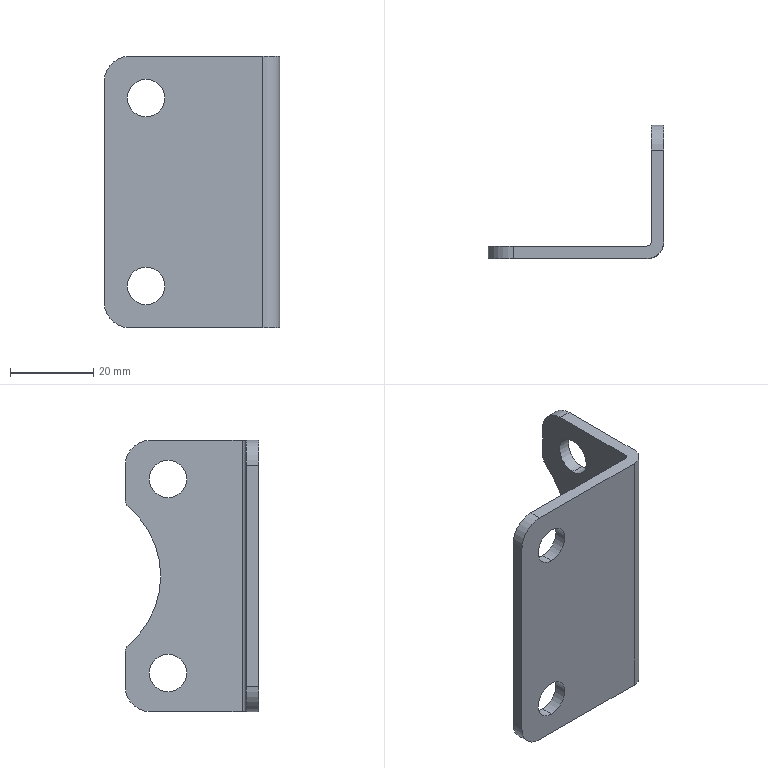Part | NX | features BREP 1 | 1 solid | 26 faces | box 42 x 32 x 65 mm | volume 12169 mm3 | cylinder 17 | plane 9 | commonest cylinder face diameters 9 x8 12 x4 4 x2 2 x1 8 x1 43 x1
STEP:
#1=CARTESIAN_POINT('',(-32.,-45.,-27.));
#2=VERTEX_POINT('',#1);
#3=CARTESIAN_POINT('',(-32.,-45.,-18.));
#4=VERTEX_POINT('',#3);
#5=CARTESIAN_POINT('',(-32.,-45.,-22.5));
#6=DIRECTION('',(0.,1.,0.));
#7=DIRECTION('',(0.,0.,1.));
#8=AXIS2_PLACEMENT_3D('',#5,#6,#7);
#9=CIRCLE('',#8,4.5);
#10=EDGE_CURVE('',#2,#4,#9,.T.);
#11=ORIENTED_EDGE('',*,*,#10,.F.);
#12=CARTESIAN_POINT('',(-32.,-42.,-27.));
#13=VERTEX_POINT('',#12);
#14=CARTESIAN_POINT('',(-32.,-42.,-27.));
#15=DIRECTION('',(0.,1.,0.));
#16=VECTOR('',#15,1000.);
#17=LINE('',#14,#16);
#18=EDGE_CURVE('',#13,#2,#17,.F.);
#19=ORIENTED_EDGE('',*,*,#18,.F.);
#20=CARTESIAN_POINT('',(-32.,-42.,-18.));
#21=VERTEX_POINT('',#20);
#22=CARTESIAN_POINT('',(-32.,-42.,-22.5));
#23=DIRECTION('',(0.,1.,0.));
#24=DIRECTION('',(0.,0.,1.));
#25=AXIS2_PLACEMENT_3D('',#22,#23,#24);
#26=CIRCLE('',#25,4.5);
#27=EDGE_CURVE('',#13,#21,#26,.T.);
#28=ORIENTED_EDGE('',*,*,#27,.T.);
#29=CARTESIAN_POINT('',(-32.,-42.,-18.));
#30=DIRECTION('',(0.,1.,0.));
#31=VECTOR('',#30,1000.);
#32=LINE('',#29,#31);
#33=EDGE_CURVE('',#21,#4,#32,.F.);
#34=ORIENTED_EDGE('',*,*,#33,.T.);
#35=EDGE_LOOP('',(#11,#19,#28,#34));
#36=FACE_BOUND('',#35,.T.);
#37=CARTESIAN_POINT('',(-32.,-42.,-22.5));
#38=DIRECTION('',(0.,1.,0.));
#39=DIRECTION('',(0.,0.,1.));
#40=AXIS2_PLACEMENT_3D('',#37,#38,#39);
#41=CYLINDRICAL_SURFACE('',#40,4.5);
#42=ADVANCED_FACE('',(#36),#41,.F.);
#43=CARTESIAN_POINT('',(-32.,-45.,18.));
#44=VERTEX_POINT('',#43);
#45=CARTESIAN_POINT('',(-32.,-45.,27.));
#46=VERTEX_POINT('',#45);
#47=CARTESIAN_POINT('',(-32.,-45.,22.5));
#48=DIRECTION('',(0.,1.,0.));
#49=DIRECTION('',(0.,0.,1.));
#50=AXIS2_PLACEMENT_3D('',#47,#48,#49);
#51=CIRCLE('',#50,4.5);
#52=EDGE_CURVE('',#44,#46,#51,.T.);
#53=ORIENTED_EDGE('',*,*,#52,.F.);
#54=CARTESIAN_POINT('',(-32.,-42.,18.));
#55=VERTEX_POINT('',#54);
#56=CARTESIAN_POINT('',(-32.,-42.,18.));
#57=DIRECTION('',(0.,1.,0.));
#58=VECTOR('',#57,1000.);
#59=LINE('',#56,#58);
#60=EDGE_CURVE('',#55,#44,#59,.F.);
#61=ORIENTED_EDGE('',*,*,#60,.F.);
#62=CARTESIAN_POINT('',(-32.,-42.,27.));
#63=VERTEX_POINT('',#62);
#64=CARTESIAN_POINT('',(-32.,-42.,22.5));
#65=DIRECTION('',(0.,1.,0.));
#66=DIRECTION('',(0.,0.,1.));
#67=AXIS2_PLACEMENT_3D('',#64,#65,#66);
#68=CIRCLE('',#67,4.5);
#69=EDGE_CURVE('',#55,#63,#68,.T.);
#70=ORIENTED_EDGE('',*,*,#69,.T.);
#71=CARTESIAN_POINT('',(-32.,-42.,27.));
#72=DIRECTION('',(0.,1.,0.));
#73=VECTOR('',#72,1000.);
#74=LINE('',#71,#73);
#75=EDGE_CURVE('',#63,#46,#74,.F.);
#76=ORIENTED_EDGE('',*,*,#75,.T.);
#77=EDGE_LOOP('',(#53,#61,#70,#76));
#78=FACE_BOUND('',#77,.T.);
#79=CARTESIAN_POINT('',(-32.,-42.,22.5));
#80=DIRECTION('',(0.,1.,0.));
#81=DIRECTION('',(0.,0.,1.));
#82=AXIS2_PLACEMENT_3D('',#79,#80,#81);
#83=CYLINDRICAL_SURFACE('',#82,4.5);
#84=ADVANCED_FACE('',(#78),#83,.F.);
#85=CARTESIAN_POINT('',(-3.,-23.25,-27.75));
#86=VERTEX_POINT('',#85);
#87=CARTESIAN_POINT('',(-3.,-23.25,-18.75));
#88=VERTEX_POINT('',#87);
#89=CARTESIAN_POINT('',(-3.,-23.25,-23.25));
#90=DIRECTION('',(-1.,0.,0.));
#91=DIRECTION('',(0.,0.,-1.));
#92=AXIS2_PLACEMENT_3D('',#89,#90,#91);
#93=CIRCLE('',#92,4.5);
#94=EDGE_CURVE('',#86,#88,#93,.T.);
#95=ORIENTED_EDGE('',*,*,#94,.T.);
#96=CARTESIAN_POINT('',(0.,-23.25,-18.75));
#97=VERTEX_POINT('',#96);
#98=CARTESIAN_POINT('',(3.,-23.25,-18.75));
#99=DIRECTION('',(1.,0.,0.));
#100=VECTOR('',#99,1000.);
#101=LINE('',#98,#100);
#102=EDGE_CURVE('',#88,#97,#101,.T.);
#103=ORIENTED_EDGE('',*,*,#102,.T.);
#104=CARTESIAN_POINT('',(0.,-23.25,-27.75));
#105=VERTEX_POINT('',#104);
#106=CARTESIAN_POINT('',(0.,-23.25,-23.25));
#107=DIRECTION('',(1.,0.,0.));
#108=DIRECTION('',(0.,0.,-1.));
#109=AXIS2_PLACEMENT_3D('',#106,#107,#108);
#110=CIRCLE('',#109,4.5);
#111=EDGE_CURVE('',#97,#105,#110,.T.);
#112=ORIENTED_EDGE('',*,*,#111,.T.);
#113=CARTESIAN_POINT('',(3.,-23.25,-27.75));
#114=DIRECTION('',(1.,0.,0.));
#115=VECTOR('',#114,1000.);
#116=LINE('',#113,#115);
#117=EDGE_CURVE('',#86,#105,#116,.T.);
#118=ORIENTED_EDGE('',*,*,#117,.F.);
#119=EDGE_LOOP('',(#95,#103,#112,#118));
#120=FACE_BOUND('',#119,.T.);
#121=CARTESIAN_POINT('',(3.,-23.25,-23.25));
#122=DIRECTION('',(1.,0.,0.));
#123=DIRECTION('',(0.,0.,-1.));
#124=AXIS2_PLACEMENT_3D('',#121,#122,#123);
#125=CYLINDRICAL_SURFACE('',#124,4.5);
#126=ADVANCED_FACE('',(#120),#125,.F.);
#127=CARTESIAN_POINT('',(-3.,-23.25,18.75));
#128=VERTEX_POINT('',#127);
#129=CARTESIAN_POINT('',(-3.,-23.25,27.75));
#130=VERTEX_POINT('',#129);
#131=CARTESIAN_POINT('',(-3.,-23.25,23.25));
#132=DIRECTION('',(-1.,0.,0.));
#133=DIRECTION('',(0.,0.,-1.));
#134=AXIS2_PLACEMENT_3D('',#131,#132,#133);
#135=CIRCLE('',#134,4.5);
#136=EDGE_CURVE('',#128,#130,#135,.T.);
#137=ORIENTED_EDGE('',*,*,#136,.T.);
#138=CARTESIAN_POINT('',(0.,-23.25,27.75));
#139=VERTEX_POINT('',#138);
#140=CARTESIAN_POINT('',(3.,-23.25,27.75));
#141=DIRECTION('',(1.,0.,0.));
#142=VECTOR('',#141,1000.);
#143=LINE('',#140,#142);
#144=EDGE_CURVE('',#130,#139,#143,.T.);
#145=ORIENTED_EDGE('',*,*,#144,.T.);
#146=CARTESIAN_POINT('',(0.,-23.25,18.75));
#147=VERTEX_POINT('',#146);
#148=CARTESIAN_POINT('',(0.,-23.25,23.25));
#149=DIRECTION('',(1.,0.,0.));
#150=DIRECTION('',(0.,0.,-1.));
#151=AXIS2_PLACEMENT_3D('',#148,#149,#150);
#152=CIRCLE('',#151,4.5);
#153=EDGE_CURVE('',#139,#147,#152,.T.);
#154=ORIENTED_EDGE('',*,*,#153,.T.);
#155=CARTESIAN_POINT('',(3.,-23.25,18.75));
#156=DIRECTION('',(1.,0.,0.));
#157=VECTOR('',#156,1000.);
#158=LINE('',#155,#157);
#159=EDGE_CURVE('',#128,#147,#158,.T.);
#160=ORIENTED_EDGE('',*,*,#159,.F.);
#161=EDGE_LOOP('',(#137,#145,#154,#160));
#162=FACE_BOUND('',#161,.T.);
#163=CARTESIAN_POINT('',(3.,-23.25,23.25));
#164=DIRECTION('',(1.,0.,0.));
#165=DIRECTION('',(0.,0.,-1.));
#166=AXIS2_PLACEMENT_3D('',#163,#164,#165);
#167=CYLINDRICAL_SURFACE('',#166,4.5);
#168=ADVANCED_FACE('',(#162),#167,.F.);
#169=CARTESIAN_POINT('',(-36.,-42.,32.5));
#170=VERTEX_POINT('',#169);
#171=CARTESIAN_POINT('',(-42.,-42.,26.5));
#172=VERTEX_POINT('',#171);
#173=CARTESIAN_POINT('',(-36.,-42.,26.5));
#174=DIRECTION('',(0.,-1.,0.));
#175=DIRECTION('',(0.,0.,1.));
#176=AXIS2_PLACEMENT_3D('',#173,#174,#175);
#177=CIRCLE('',#176,6.);
#178=EDGE_CURVE('',#170,#172,#177,.T.);
#179=ORIENTED_EDGE('',*,*,#178,.F.);
#180=CARTESIAN_POINT('',(-4.,-42.,32.5));
#181=VERTEX_POINT('',#180);
#182=CARTESIAN_POINT('',(-4.,-42.,32.5));
#183=DIRECTION('',(-1.,0.,0.));
#184=VECTOR('',#183,1000.);
#185=LINE('',#182,#184);
#186=EDGE_CURVE('',#181,#170,#185,.T.);
#187=ORIENTED_EDGE('',*,*,#186,.F.);
#188=CARTESIAN_POINT('',(-4.,-42.,-32.5));
#189=VERTEX_POINT('',#188);
#190=CARTESIAN_POINT('',(-4.,-42.,32.5));
#191=DIRECTION('',(0.,0.,1.));
#192=VECTOR('',#191,1000.);
#193=LINE('',#190,#192);
#194=EDGE_CURVE('',#189,#181,#193,.T.);
#195=ORIENTED_EDGE('',*,*,#194,.F.);
#196=CARTESIAN_POINT('',(-36.,-42.,-32.5));
#197=VERTEX_POINT('',#196);
#198=CARTESIAN_POINT('',(-4.,-42.,-32.5));
#199=DIRECTION('',(1.,0.,0.));
#200=VECTOR('',#199,1000.);
#201=LINE('',#198,#200);
#202=EDGE_CURVE('',#197,#189,#201,.T.);
#203=ORIENTED_EDGE('',*,*,#202,.F.);
#204=CARTESIAN_POINT('',(-42.,-42.,-26.5));
#205=VERTEX_POINT('',#204);
#206=CARTESIAN_POINT('',(-36.,-42.,-26.5));
#207=DIRECTION('',(0.,-1.,0.));
#208=DIRECTION('',(0.,0.,1.));
#209=AXIS2_PLACEMENT_3D('',#206,#207,#208);
#210=CIRCLE('',#209,6.);
#211=EDGE_CURVE('',#205,#197,#210,.T.);
#212=ORIENTED_EDGE('',*,*,#211,.F.);
#213=CARTESIAN_POINT('',(-42.,-42.,32.5));
#214=DIRECTION('',(0.,0.,-1.));
#215=VECTOR('',#214,1000.);
#216=LINE('',#213,#215);
#217=EDGE_CURVE('',#172,#205,#216,.T.);
#218=ORIENTED_EDGE('',*,*,#217,.F.);
#219=EDGE_LOOP('',(#179,#187,#195,#203,#212,#218));
#220=FACE_BOUND('',#219,.T.);
#221=CARTESIAN_POINT('',(-32.,-42.,-22.5));
#222=DIRECTION('',(0.,1.,0.));
#223=DIRECTION('',(0.,0.,1.));
#224=AXIS2_PLACEMENT_3D('',#221,#222,#223);
#225=CIRCLE('',#224,4.5);
#226=EDGE_CURVE('',#21,#13,#225,.T.);
#227=ORIENTED_EDGE('',*,*,#226,.F.);
#228=ORIENTED_EDGE('',*,*,#27,.F.);
#229=EDGE_LOOP('',(#227,#228));
#230=FACE_BOUND('',#229,.T.);
#231=CARTESIAN_POINT('',(-32.,-42.,22.5));
#232=DIRECTION('',(0.,1.,0.));
#233=DIRECTION('',(0.,0.,1.));
#234=AXIS2_PLACEMENT_3D('',#231,#232,#233);
#235=CIRCLE('',#234,4.5);
#236=EDGE_CURVE('',#63,#55,#235,.T.);
#237=ORIENTED_EDGE('',*,*,#236,.F.);
#238=ORIENTED_EDGE('',*,*,#69,.F.);
#239=EDGE_LOOP('',(#237,#238));
#240=FACE_BOUND('',#239,.T.);
#241=CARTESIAN_POINT('',(-4.,-42.,32.5));
#242=DIRECTION('',(0.,-1.,0.));
#243=DIRECTION('',(0.,0.,-1.));
#244=AXIS2_PLACEMENT_3D('',#241,#242,#243);
#245=PLANE('',#244);
#246=ADVANCED_FACE('',(#220,#230,#240),#245,.F.);
#247=CARTESIAN_POINT('',(-42.,-45.,26.5));
#248=VERTEX_POINT('',#247);
#249=CARTESIAN_POINT('',(-42.,-42.,26.5));
#250=DIRECTION('',(0.,-1.,0.));
#251=VECTOR('',#250,1000.);
#252=LINE('',#249,#251);
#253=EDGE_CURVE('',#172,#248,#252,.T.);
#254=ORIENTED_EDGE('',*,*,#253,.F.);
#255=ORIENTED_EDGE('',*,*,#217,.T.);
#256=CARTESIAN_POINT('',(-42.,-45.,-26.5));
#257=VERTEX_POINT('',#256);
#258=CARTESIAN_POINT('',(-42.,-42.,-26.5));
#259=DIRECTION('',(0.,1.,0.));
#260=VECTOR('',#259,1000.);
#261=LINE('',#258,#260);
#262=EDGE_CURVE('',#257,#205,#261,.T.);
#263=ORIENTED_EDGE('',*,*,#262,.F.);
#264=CARTESIAN_POINT('',(-42.,-45.,32.5));
#265=DIRECTION('',(0.,0.,-1.));
#266=VECTOR('',#265,1000.);
#267=LINE('',#264,#266);
#268=EDGE_CURVE('',#248,#257,#267,.T.);
#269=ORIENTED_EDGE('',*,*,#268,.F.);
#270=EDGE_LOOP('',(#254,#255,#263,#269));
#271=FACE_BOUND('',#270,.T.);
#272=CARTESIAN_POINT('',(-42.,-42.,32.5));
#273=DIRECTION('',(1.,0.,0.));
#274=DIRECTION('',(0.,1.,0.));
#275=AXIS2_PLACEMENT_3D('',#272,#273,#274);
#276=PLANE('',#275);
#277=ADVANCED_FACE('',(#271),#276,.F.);
#278=ORIENTED_EDGE('',*,*,#253,.T.);
#279=CARTESIAN_POINT('',(-36.,-45.,32.5));
#280=VERTEX_POINT('',#279);
#281=CARTESIAN_POINT('',(-36.,-45.,26.5));
#282=DIRECTION('',(0.,1.,0.));
#283=DIRECTION('',(0.,0.,1.));
#284=AXIS2_PLACEMENT_3D('',#281,#282,#283);
#285=CIRCLE('',#284,6.);
#286=EDGE_CURVE('',#248,#280,#285,.T.);
#287=ORIENTED_EDGE('',*,*,#286,.T.);
#288=CARTESIAN_POINT('',(-36.,-42.,32.5));
#289=DIRECTION('',(0.,1.,0.));
#290=VECTOR('',#289,1000.);
#291=LINE('',#288,#290);
#292=EDGE_CURVE('',#280,#170,#291,.T.);
#293=ORIENTED_EDGE('',*,*,#292,.T.);
#294=ORIENTED_EDGE('',*,*,#178,.T.);
#295=EDGE_LOOP('',(#278,#287,#293,#294));
#296=FACE_BOUND('',#295,.T.);
#297=CARTESIAN_POINT('',(-36.,-42.,26.5));
#298=DIRECTION('',(0.,1.,0.));
#299=DIRECTION('',(0.,0.,1.));
#300=AXIS2_PLACEMENT_3D('',#297,#298,#299);
#301=CYLINDRICAL_SURFACE('',#300,6.);
#302=ADVANCED_FACE('',(#296),#301,.T.);
#303=ORIENTED_EDGE('',*,*,#186,.T.);
#304=ORIENTED_EDGE('',*,*,#292,.F.);
#305=CARTESIAN_POINT('',(-4.,-45.,32.5));
#306=VERTEX_POINT('',#305);
#307=CARTESIAN_POINT('',(-4.,-45.,32.5));
#308=DIRECTION('',(1.,0.,0.));
#309=VECTOR('',#308,1000.);
#310=LINE('',#307,#309);
#311=EDGE_CURVE('',#280,#306,#310,.T.);
#312=ORIENTED_EDGE('',*,*,#311,.T.);
#313=CARTESIAN_POINT('',(0.,-41.,32.5));
#314=VERTEX_POINT('',#313);
#315=CARTESIAN_POINT('',(-4.,-41.,32.5));
#316=DIRECTION('',(0.,0.,1.));
#317=DIRECTION('',(1.,0.,0.));
#318=AXIS2_PLACEMENT_3D('',#315,#316,#317);
#319=CIRCLE('',#318,4.);
#320=EDGE_CURVE('',#306,#314,#319,.T.);
#321=ORIENTED_EDGE('',*,*,#320,.T.);
#322=CARTESIAN_POINT('',(0.,-19.,32.5));
#323=VERTEX_POINT('',#322);
#324=CARTESIAN_POINT('',(0.,-41.,32.5));
#325=DIRECTION('',(0.,1.,0.));
#326=VECTOR('',#325,1000.);
#327=LINE('',#324,#326);
#328=EDGE_CURVE('',#314,#323,#327,.T.);
#329=ORIENTED_EDGE('',*,*,#328,.T.);
#330=CARTESIAN_POINT('',(-3.,-19.,32.5));
#331=VERTEX_POINT('',#330);
#332=CARTESIAN_POINT('',(-4.,-19.,32.5));
#333=DIRECTION('',(-1.,0.,0.));
#334=VECTOR('',#333,1000.);
#335=LINE('',#332,#334);
#336=EDGE_CURVE('',#323,#331,#335,.T.);
#337=ORIENTED_EDGE('',*,*,#336,.T.);
#338=CARTESIAN_POINT('',(-3.,-41.,32.5));
#339=VERTEX_POINT('',#338);
#340=CARTESIAN_POINT('',(-3.,-41.,32.5));
#341=DIRECTION('',(0.,-1.,0.));
#342=VECTOR('',#341,1000.);
#343=LINE('',#340,#342);
#344=EDGE_CURVE('',#331,#339,#343,.T.);
#345=ORIENTED_EDGE('',*,*,#344,.T.);
#346=CARTESIAN_POINT('',(-4.,-41.,32.5));
#347=DIRECTION('',(0.,0.,-1.));
#348=DIRECTION('',(1.,0.,0.));
#349=AXIS2_PLACEMENT_3D('',#346,#347,#348);
#350=CIRCLE('',#349,1.);
#351=EDGE_CURVE('',#339,#181,#350,.T.);
#352=ORIENTED_EDGE('',*,*,#351,.T.);
#353=EDGE_LOOP('',(#303,#304,#312,#321,#329,#337,#345,#352));
#354=FACE_BOUND('',#353,.T.);
#355=CARTESIAN_POINT('',(-4.,-41.,32.5));
#356=DIRECTION('',(0.,0.,1.));
#357=DIRECTION('',(1.,0.,0.));
#358=AXIS2_PLACEMENT_3D('',#355,#356,#357);
#359=PLANE('',#358);
#360=ADVANCED_FACE('',(#354),#359,.T.);
#361=ORIENTED_EDGE('',*,*,#194,.T.);
#362=ORIENTED_EDGE('',*,*,#351,.F.);
#363=CARTESIAN_POINT('',(-3.,-41.,-32.5));
#364=VERTEX_POINT('',#363);
#365=CARTESIAN_POINT('',(-3.,-41.,32.5));
#366=DIRECTION('',(0.,0.,1.));
#367=VECTOR('',#366,1000.);
#368=LINE('',#365,#367);
#369=EDGE_CURVE('',#364,#339,#368,.T.);
#370=ORIENTED_EDGE('',*,*,#369,.F.);
#371=CARTESIAN_POINT('',(-4.,-41.,-32.5));
#372=DIRECTION('',(0.,0.,1.));
#373=DIRECTION('',(1.,0.,0.));
#374=AXIS2_PLACEMENT_3D('',#371,#372,#373);
#375=CIRCLE('',#374,1.);
#376=EDGE_CURVE('',#189,#364,#375,.T.);
#377=ORIENTED_EDGE('',*,*,#376,.F.);
#378=EDGE_LOOP('',(#361,#362,#370,#377));
#379=FACE_BOUND('',#378,.T.);
#380=CARTESIAN_POINT('',(-4.,-41.,32.5));
#381=DIRECTION('',(0.,0.,1.));
#382=DIRECTION('',(1.,0.,0.));
#383=AXIS2_PLACEMENT_3D('',#380,#381,#382);
#384=CYLINDRICAL_SURFACE('',#383,1.);
#385=ADVANCED_FACE('',(#379),#384,.F.);
#386=CARTESIAN_POINT('',(-36.,-45.,-32.5));
#387=VERTEX_POINT('',#386);
#388=CARTESIAN_POINT('',(-36.,-41.,-32.5));
#389=DIRECTION('',(0.,-1.,0.));
#390=VECTOR('',#389,1000.);
#391=LINE('',#388,#390);
#392=EDGE_CURVE('',#197,#387,#391,.T.);
#393=ORIENTED_EDGE('',*,*,#392,.F.);
#394=ORIENTED_EDGE('',*,*,#202,.T.);
#395=ORIENTED_EDGE('',*,*,#376,.T.);
#396=CARTESIAN_POINT('',(-3.,-19.,-32.5));
#397=VERTEX_POINT('',#396);
#398=CARTESIAN_POINT('',(-3.,-41.,-32.5));
#399=DIRECTION('',(0.,-1.,0.));
#400=VECTOR('',#399,1000.);
#401=LINE('',#398,#400);
#402=EDGE_CURVE('',#397,#364,#401,.T.);
#403=ORIENTED_EDGE('',*,*,#402,.F.);
#404=CARTESIAN_POINT('',(0.,-19.,-32.5));
#405=VERTEX_POINT('',#404);
#406=CARTESIAN_POINT('',(-4.,-19.,-32.5));
#407=DIRECTION('',(-1.,0.,0.));
#408=VECTOR('',#407,1000.);
#409=LINE('',#406,#408);
#410=EDGE_CURVE('',#405,#397,#409,.T.);
#411=ORIENTED_EDGE('',*,*,#410,.F.);
#412=CARTESIAN_POINT('',(0.,-41.,-32.5));
#413=VERTEX_POINT('',#412);
#414=CARTESIAN_POINT('',(0.,-41.,-32.5));
#415=DIRECTION('',(0.,1.,0.));
#416=VECTOR('',#415,1000.);
#417=LINE('',#414,#416);
#418=EDGE_CURVE('',#413,#405,#417,.T.);
#419=ORIENTED_EDGE('',*,*,#418,.F.);
#420=CARTESIAN_POINT('',(-4.,-45.,-32.5));
#421=VERTEX_POINT('',#420);
#422=CARTESIAN_POINT('',(-4.,-41.,-32.5));
#423=DIRECTION('',(0.,0.,1.));
#424=DIRECTION('',(1.,0.,0.));
#425=AXIS2_PLACEMENT_3D('',#422,#423,#424);
#426=CIRCLE('',#425,4.);
#427=EDGE_CURVE('',#421,#413,#426,.T.);
#428=ORIENTED_EDGE('',*,*,#427,.F.);
#429=CARTESIAN_POINT('',(-4.,-45.,-32.5));
#430=DIRECTION('',(1.,0.,0.));
#431=VECTOR('',#430,1000.);
#432=LINE('',#429,#431);
#433=EDGE_CURVE('',#387,#421,#432,.T.);
#434=ORIENTED_EDGE('',*,*,#433,.F.);
#435=EDGE_LOOP('',(#393,#394,#395,#403,#411,#419,#428,#434));
#436=FACE_BOUND('',#435,.T.);
#437=CARTESIAN_POINT('',(-4.,-41.,-32.5));
#438=DIRECTION('',(0.,0.,1.));
#439=DIRECTION('',(1.,0.,0.));
#440=AXIS2_PLACEMENT_3D('',#437,#438,#439);
#441=PLANE('',#440);
#442=ADVANCED_FACE('',(#436),#441,.F.);
#443=ORIENTED_EDGE('',*,*,#392,.T.);
#444=CARTESIAN_POINT('',(-36.,-45.,-26.5));
#445=DIRECTION('',(0.,1.,0.));
#446=DIRECTION('',(0.,0.,1.));
#447=AXIS2_PLACEMENT_3D('',#444,#445,#446);
#448=CIRCLE('',#447,6.);
#449=EDGE_CURVE('',#387,#257,#448,.T.);
#450=ORIENTED_EDGE('',*,*,#449,.T.);
#451=ORIENTED_EDGE('',*,*,#262,.T.);
#452=ORIENTED_EDGE('',*,*,#211,.T.);
#453=EDGE_LOOP('',(#443,#450,#451,#452));
#454=FACE_BOUND('',#453,.T.);
#455=CARTESIAN_POINT('',(-36.,-42.,-26.5));
#456=DIRECTION('',(0.,1.,0.));
#457=DIRECTION('',(0.,0.,1.));
#458=AXIS2_PLACEMENT_3D('',#455,#456,#457);
#459=CYLINDRICAL_SURFACE('',#458,6.);
#460=ADVANCED_FACE('',(#454),#459,.T.);
#461=ORIENTED_EDGE('',*,*,#18,.T.);
#462=CARTESIAN_POINT('',(-32.,-45.,-22.5));
#463=DIRECTION('',(0.,1.,0.));
#464=DIRECTION('',(0.,0.,1.));
#465=AXIS2_PLACEMENT_3D('',#462,#463,#464);
#466=CIRCLE('',#465,4.5);
#467=EDGE_CURVE('',#4,#2,#466,.T.);
#468=ORIENTED_EDGE('',*,*,#467,.F.);
#469=ORIENTED_EDGE('',*,*,#33,.F.);
#470=ORIENTED_EDGE('',*,*,#226,.T.);
#471=EDGE_LOOP('',(#461,#468,#469,#470));
#472=FACE_BOUND('',#471,.T.);
#473=CARTESIAN_POINT('',(-32.,-42.,-22.5));
#474=DIRECTION('',(0.,1.,0.));
#475=DIRECTION('',(0.,0.,1.));
#476=AXIS2_PLACEMENT_3D('',#473,#474,#475);
#477=CYLINDRICAL_SURFACE('',#476,4.5);
#478=ADVANCED_FACE('',(#472),#477,.F.);
#479=ORIENTED_EDGE('',*,*,#60,.T.);
#480=CARTESIAN_POINT('',(-32.,-45.,22.5));
#481=DIRECTION('',(0.,1.,0.));
#482=DIRECTION('',(0.,0.,1.));
#483=AXIS2_PLACEMENT_3D('',#480,#481,#482);
#484=CIRCLE('',#483,4.5);
#485=EDGE_CURVE('',#46,#44,#484,.T.);
#486=ORIENTED_EDGE('',*,*,#485,.F.);
#487=ORIENTED_EDGE('',*,*,#75,.F.);
#488=ORIENTED_EDGE('',*,*,#236,.T.);
#489=EDGE_LOOP('',(#479,#486,#487,#488));
#490=FACE_BOUND('',#489,.T.);
#491=CARTESIAN_POINT('',(-32.,-42.,22.5));
#492=DIRECTION('',(0.,1.,0.));
#493=DIRECTION('',(0.,0.,1.));
#494=AXIS2_PLACEMENT_3D('',#491,#492,#493);
#495=CYLINDRICAL_SURFACE('',#494,4.5);
#496=ADVANCED_FACE('',(#490),#495,.F.);
#497=ORIENTED_EDGE('',*,*,#286,.F.);
#498=ORIENTED_EDGE('',*,*,#268,.T.);
#499=ORIENTED_EDGE('',*,*,#449,.F.);
#500=ORIENTED_EDGE('',*,*,#433,.T.);
#501=CARTESIAN_POINT('',(-4.,-45.,32.5));
#502=DIRECTION('',(0.,0.,-1.));
#503=VECTOR('',#502,1000.);
#504=LINE('',#501,#503);
#505=EDGE_CURVE('',#306,#421,#504,.T.);
#506=ORIENTED_EDGE('',*,*,#505,.F.);
#507=ORIENTED_EDGE('',*,*,#311,.F.);
#508=EDGE_LOOP('',(#497,#498,#499,#500,#506,#507));
#509=FACE_BOUND('',#508,.T.);
#510=ORIENTED_EDGE('',*,*,#467,.T.);
#511=ORIENTED_EDGE('',*,*,#10,.T.);
#512=EDGE_LOOP('',(#510,#511));
#513=FACE_BOUND('',#512,.T.);
#514=ORIENTED_EDGE('',*,*,#485,.T.);
#515=ORIENTED_EDGE('',*,*,#52,.T.);
#516=EDGE_LOOP('',(#514,#515));
#517=FACE_BOUND('',#516,.T.);
#518=CARTESIAN_POINT('',(-42.,-45.,32.5));
#519=DIRECTION('',(0.,1.,0.));
#520=DIRECTION('',(1.,0.,0.));
#521=AXIS2_PLACEMENT_3D('',#518,#519,#520);
#522=PLANE('',#521);
#523=ADVANCED_FACE('',(#509,#513,#517),#522,.F.);
#524=CARTESIAN_POINT('',(-3.,-13.,26.5));
#525=VERTEX_POINT('',#524);
#526=CARTESIAN_POINT('',(-3.,-19.,26.5));
#527=DIRECTION('',(1.,0.,0.));
#528=DIRECTION('',(0.,0.,-1.));
#529=AXIS2_PLACEMENT_3D('',#526,#527,#528);
#530=CIRCLE('',#529,6.);
#531=EDGE_CURVE('',#525,#331,#530,.T.);
#532=ORIENTED_EDGE('',*,*,#531,.F.);
#533=CARTESIAN_POINT('',(-3.,-13.,18.09));
#534=VERTEX_POINT('',#533);
#535=CARTESIAN_POINT('',(-3.,-13.,32.5));
#536=DIRECTION('',(0.,0.,1.));
#537=VECTOR('',#536,1000.);
#538=LINE('',#535,#537);
#539=EDGE_CURVE('',#534,#525,#538,.T.);
#540=ORIENTED_EDGE('',*,*,#539,.F.);
#541=CARTESIAN_POINT('',(-3.,-13.723,16.55));
#542=VERTEX_POINT('',#541);
#543=CARTESIAN_POINT('',(-3.,-15.,18.09));
#544=DIRECTION('',(1.,0.,0.));
#545=DIRECTION('',(0.,0.,-1.));
#546=AXIS2_PLACEMENT_3D('',#543,#544,#545);
#547=CIRCLE('',#546,2.);
#548=EDGE_CURVE('',#542,#534,#547,.T.);
#549=ORIENTED_EDGE('',*,*,#548,.F.);
#550=CARTESIAN_POINT('',(-3.,-13.723,-16.55));
#551=VERTEX_POINT('',#550);
#552=CARTESIAN_POINT('',(-3.,0.,0.));
#553=DIRECTION('',(-1.,0.,0.));
#554=DIRECTION('',(0.,0.,-1.));
#555=AXIS2_PLACEMENT_3D('',#552,#553,#554);
#556=CIRCLE('',#555,21.5);
#557=EDGE_CURVE('',#551,#542,#556,.T.);
#558=ORIENTED_EDGE('',*,*,#557,.F.);
#559=CARTESIAN_POINT('',(-3.,-13.,-18.09));
#560=VERTEX_POINT('',#559);
#561=CARTESIAN_POINT('',(-3.,-15.,-18.09));
#562=DIRECTION('',(1.,0.,0.));
#563=DIRECTION('',(0.,0.,-1.));
#564=AXIS2_PLACEMENT_3D('',#561,#562,#563);
#565=CIRCLE('',#564,2.);
#566=EDGE_CURVE('',#560,#551,#565,.T.);
#567=ORIENTED_EDGE('',*,*,#566,.F.);
#568=CARTESIAN_POINT('',(-3.,-13.,-26.5));
#569=VERTEX_POINT('',#568);
#570=CARTESIAN_POINT('',(-3.,-13.,32.5));
#571=DIRECTION('',(0.,0.,1.));
#572=VECTOR('',#571,1000.);
#573=LINE('',#570,#572);
#574=EDGE_CURVE('',#569,#560,#573,.T.);
#575=ORIENTED_EDGE('',*,*,#574,.F.);
#576=CARTESIAN_POINT('',(-3.,-19.,-26.5));
#577=DIRECTION('',(1.,0.,0.));
#578=DIRECTION('',(0.,0.,-1.));
#579=AXIS2_PLACEMENT_3D('',#576,#577,#578);
#580=CIRCLE('',#579,6.);
#581=EDGE_CURVE('',#397,#569,#580,.T.);
#582=ORIENTED_EDGE('',*,*,#581,.F.);
#583=ORIENTED_EDGE('',*,*,#402,.T.);
#584=ORIENTED_EDGE('',*,*,#369,.T.);
#585=ORIENTED_EDGE('',*,*,#344,.F.);
#586=EDGE_LOOP('',(#532,#540,#549,#558,#567,#575,#582,#583,#584,#585));
#587=FACE_BOUND('',#586,.T.);
#588=ORIENTED_EDGE('',*,*,#94,.F.);
#589=CARTESIAN_POINT('',(-3.,-23.25,-23.25));
#590=DIRECTION('',(-1.,0.,0.));
#591=DIRECTION('',(0.,0.,-1.));
#592=AXIS2_PLACEMENT_3D('',#589,#590,#591);
#593=CIRCLE('',#592,4.5);
#594=EDGE_CURVE('',#88,#86,#593,.T.);
#595=ORIENTED_EDGE('',*,*,#594,.F.);
#596=EDGE_LOOP('',(#588,#595));
#597=FACE_BOUND('',#596,.T.);
#598=ORIENTED_EDGE('',*,*,#136,.F.);
#599=CARTESIAN_POINT('',(-3.,-23.25,23.25));
#600=DIRECTION('',(-1.,0.,0.));
#601=DIRECTION('',(0.,0.,-1.));
#602=AXIS2_PLACEMENT_3D('',#599,#600,#601);
#603=CIRCLE('',#602,4.5);
#604=EDGE_CURVE('',#130,#128,#603,.T.);
#605=ORIENTED_EDGE('',*,*,#604,.F.);
#606=EDGE_LOOP('',(#598,#605));
#607=FACE_BOUND('',#606,.T.);
#608=CARTESIAN_POINT('',(-3.,-13.,32.5));
#609=DIRECTION('',(1.,0.,0.));
#610=DIRECTION('',(0.,1.,0.));
#611=AXIS2_PLACEMENT_3D('',#608,#609,#610);
#612=PLANE('',#611);
#613=ADVANCED_FACE('',(#587,#597,#607),#612,.F.);
#614=ORIENTED_EDGE('',*,*,#336,.F.);
#615=CARTESIAN_POINT('',(0.,-13.,26.5));
#616=VERTEX_POINT('',#615);
#617=CARTESIAN_POINT('',(0.,-19.,26.5));
#618=DIRECTION('',(-1.,0.,0.));
#619=DIRECTION('',(0.,0.,-1.));
#620=AXIS2_PLACEMENT_3D('',#617,#618,#619);
#621=CIRCLE('',#620,6.);
#622=EDGE_CURVE('',#323,#616,#621,.T.);
#623=ORIENTED_EDGE('',*,*,#622,.T.);
#624=CARTESIAN_POINT('',(3.,-13.,26.5));
#625=DIRECTION('',(-1.,0.,0.));
#626=VECTOR('',#625,1000.);
#627=LINE('',#624,#626);
#628=EDGE_CURVE('',#616,#525,#627,.T.);
#629=ORIENTED_EDGE('',*,*,#628,.T.);
#630=ORIENTED_EDGE('',*,*,#531,.T.);
#631=EDGE_LOOP('',(#614,#623,#629,#630));
#632=FACE_BOUND('',#631,.T.);
#633=CARTESIAN_POINT('',(3.,-19.,26.5));
#634=DIRECTION('',(1.,0.,0.));
#635=DIRECTION('',(0.,0.,-1.));
#636=AXIS2_PLACEMENT_3D('',#633,#634,#635);
#637=CYLINDRICAL_SURFACE('',#636,6.);
#638=ADVANCED_FACE('',(#632),#637,.T.);
#639=ORIENTED_EDGE('',*,*,#622,.F.);
#640=ORIENTED_EDGE('',*,*,#328,.F.);
#641=CARTESIAN_POINT('',(0.,-41.,32.5));
#642=DIRECTION('',(0.,0.,1.));
#643=VECTOR('',#642,1000.);
#644=LINE('',#641,#643);
#645=EDGE_CURVE('',#413,#314,#644,.T.);
#646=ORIENTED_EDGE('',*,*,#645,.F.);
#647=ORIENTED_EDGE('',*,*,#418,.T.);
#648=CARTESIAN_POINT('',(0.,-13.,-26.5));
#649=VERTEX_POINT('',#648);
#650=CARTESIAN_POINT('',(0.,-19.,-26.5));
#651=DIRECTION('',(-1.,0.,0.));
#652=DIRECTION('',(0.,0.,-1.));
#653=AXIS2_PLACEMENT_3D('',#650,#651,#652);
#654=CIRCLE('',#653,6.);
#655=EDGE_CURVE('',#649,#405,#654,.T.);
#656=ORIENTED_EDGE('',*,*,#655,.F.);
#657=CARTESIAN_POINT('',(0.,-13.,-18.09));
#658=VERTEX_POINT('',#657);
#659=CARTESIAN_POINT('',(0.,-13.,32.5));
#660=DIRECTION('',(0.,0.,-1.));
#661=VECTOR('',#660,1000.);
#662=LINE('',#659,#661);
#663=EDGE_CURVE('',#658,#649,#662,.T.);
#664=ORIENTED_EDGE('',*,*,#663,.F.);
#665=CARTESIAN_POINT('',(0.,-13.723,-16.55));
#666=VERTEX_POINT('',#665);
#667=CARTESIAN_POINT('',(0.,-15.,-18.09));
#668=DIRECTION('',(-1.,0.,0.));
#669=DIRECTION('',(0.,0.,-1.));
#670=AXIS2_PLACEMENT_3D('',#667,#668,#669);
#671=CIRCLE('',#670,2.);
#672=EDGE_CURVE('',#666,#658,#671,.T.);
#673=ORIENTED_EDGE('',*,*,#672,.F.);
#674=CARTESIAN_POINT('',(0.,-13.723,16.55));
#675=VERTEX_POINT('',#674);
#676=CARTESIAN_POINT('',(0.,0.,0.));
#677=DIRECTION('',(1.,0.,0.));
#678=DIRECTION('',(0.,0.,-1.));
#679=AXIS2_PLACEMENT_3D('',#676,#677,#678);
#680=CIRCLE('',#679,21.5);
#681=EDGE_CURVE('',#675,#666,#680,.T.);
#682=ORIENTED_EDGE('',*,*,#681,.F.);
#683=CARTESIAN_POINT('',(0.,-13.,18.09));
#684=VERTEX_POINT('',#683);
#685=CARTESIAN_POINT('',(0.,-15.,18.09));
#686=DIRECTION('',(-1.,0.,0.));
#687=DIRECTION('',(0.,0.,-1.));
#688=AXIS2_PLACEMENT_3D('',#685,#686,#687);
#689=CIRCLE('',#688,2.);
#690=EDGE_CURVE('',#684,#675,#689,.T.);
#691=ORIENTED_EDGE('',*,*,#690,.F.);
#692=CARTESIAN_POINT('',(0.,-13.,32.5));
#693=DIRECTION('',(0.,0.,-1.));
#694=VECTOR('',#693,1000.);
#695=LINE('',#692,#694);
#696=EDGE_CURVE('',#616,#684,#695,.T.);
#697=ORIENTED_EDGE('',*,*,#696,.F.);
#698=EDGE_LOOP('',(#639,#640,#646,#647,#656,#664,#673,#682,#691,#697));
#699=FACE_BOUND('',#698,.T.);
#700=CARTESIAN_POINT('',(0.,-23.25,-23.25));
#701=DIRECTION('',(1.,0.,0.));
#702=DIRECTION('',(0.,0.,-1.));
#703=AXIS2_PLACEMENT_3D('',#700,#701,#702);
#704=CIRCLE('',#703,4.5);
#705=EDGE_CURVE('',#105,#97,#704,.T.);
#706=ORIENTED_EDGE('',*,*,#705,.F.);
#707=ORIENTED_EDGE('',*,*,#111,.F.);
#708=EDGE_LOOP('',(#706,#707));
#709=FACE_BOUND('',#708,.T.);
#710=CARTESIAN_POINT('',(0.,-23.25,23.25));
#711=DIRECTION('',(1.,0.,0.));
#712=DIRECTION('',(0.,0.,-1.));
#713=AXIS2_PLACEMENT_3D('',#710,#711,#712);
#714=CIRCLE('',#713,4.5);
#715=EDGE_CURVE('',#147,#139,#714,.T.);
#716=ORIENTED_EDGE('',*,*,#715,.F.);
#717=ORIENTED_EDGE('',*,*,#153,.F.);
#718=EDGE_LOOP('',(#716,#717));
#719=FACE_BOUND('',#718,.T.);
#720=CARTESIAN_POINT('',(0.,-41.,32.5));
#721=DIRECTION('',(-1.,0.,0.));
#722=DIRECTION('',(0.,0.,1.));
#723=AXIS2_PLACEMENT_3D('',#720,#721,#722);
#724=PLANE('',#723);
#725=ADVANCED_FACE('',(#699,#709,#719),#724,.F.);
#726=ORIENTED_EDGE('',*,*,#320,.F.);
#727=ORIENTED_EDGE('',*,*,#505,.T.);
#728=ORIENTED_EDGE('',*,*,#427,.T.);
#729=ORIENTED_EDGE('',*,*,#645,.T.);
#730=EDGE_LOOP('',(#726,#727,#728,#729));
#731=FACE_BOUND('',#730,.T.);
#732=CARTESIAN_POINT('',(-4.,-41.,32.5));
#733=DIRECTION('',(0.,0.,1.));
#734=DIRECTION('',(1.,0.,0.));
#735=AXIS2_PLACEMENT_3D('',#732,#733,#734);
#736=CYLINDRICAL_SURFACE('',#735,4.);
#737=ADVANCED_FACE('',(#731),#736,.T.);
#738=CARTESIAN_POINT('',(3.,-13.,-26.5));
#739=DIRECTION('',(1.,0.,0.));
#740=VECTOR('',#739,1000.);
#741=LINE('',#738,#740);
#742=EDGE_CURVE('',#569,#649,#741,.T.);
#743=ORIENTED_EDGE('',*,*,#742,.T.);
#744=ORIENTED_EDGE('',*,*,#655,.T.);
#745=ORIENTED_EDGE('',*,*,#410,.T.);
#746=ORIENTED_EDGE('',*,*,#581,.T.);
#747=EDGE_LOOP('',(#743,#744,#745,#746));
#748=FACE_BOUND('',#747,.T.);
#749=CARTESIAN_POINT('',(3.,-19.,-26.5));
#750=DIRECTION('',(1.,0.,0.));
#751=DIRECTION('',(0.,0.,-1.));
#752=AXIS2_PLACEMENT_3D('',#749,#750,#751);
#753=CYLINDRICAL_SURFACE('',#752,6.);
#754=ADVANCED_FACE('',(#748),#753,.T.);
#755=ORIENTED_EDGE('',*,*,#628,.F.);
#756=ORIENTED_EDGE('',*,*,#696,.T.);
#757=CARTESIAN_POINT('',(0.,-13.,18.09));
#758=DIRECTION('',(1.,0.,0.));
#759=VECTOR('',#758,1000.);
#760=LINE('',#757,#759);
#761=EDGE_CURVE('',#534,#684,#760,.T.);
#762=ORIENTED_EDGE('',*,*,#761,.F.);
#763=ORIENTED_EDGE('',*,*,#539,.T.);
#764=EDGE_LOOP('',(#755,#756,#762,#763));
#765=FACE_BOUND('',#764,.T.);
#766=CARTESIAN_POINT('',(0.,-13.,32.5));
#767=DIRECTION('',(0.,-1.,0.));
#768=DIRECTION('',(0.,0.,-1.));
#769=AXIS2_PLACEMENT_3D('',#766,#767,#768);
#770=PLANE('',#769);
#771=ADVANCED_FACE('',(#765),#770,.F.);
#772=ORIENTED_EDGE('',*,*,#761,.T.);
#773=ORIENTED_EDGE('',*,*,#690,.T.);
#774=CARTESIAN_POINT('',(3.,-13.723,16.55));
#775=DIRECTION('',(-1.,0.,0.));
#776=VECTOR('',#775,1000.);
#777=LINE('',#774,#776);
#778=EDGE_CURVE('',#675,#542,#777,.T.);
#779=ORIENTED_EDGE('',*,*,#778,.T.);
#780=ORIENTED_EDGE('',*,*,#548,.T.);
#781=EDGE_LOOP('',(#772,#773,#779,#780));
#782=FACE_BOUND('',#781,.T.);
#783=CARTESIAN_POINT('',(3.,-15.,18.09));
#784=DIRECTION('',(1.,0.,0.));
#785=DIRECTION('',(0.,0.,-1.));
#786=AXIS2_PLACEMENT_3D('',#783,#784,#785);
#787=CYLINDRICAL_SURFACE('',#786,2.);
#788=ADVANCED_FACE('',(#782),#787,.T.);
#789=CARTESIAN_POINT('',(3.,-13.723,-16.55));
#790=DIRECTION('',(1.,0.,0.));
#791=VECTOR('',#790,1000.);
#792=LINE('',#789,#791);
#793=EDGE_CURVE('',#551,#666,#792,.T.);
#794=ORIENTED_EDGE('',*,*,#793,.F.);
#795=ORIENTED_EDGE('',*,*,#557,.T.);
#796=ORIENTED_EDGE('',*,*,#778,.F.);
#797=ORIENTED_EDGE('',*,*,#681,.T.);
#798=EDGE_LOOP('',(#794,#795,#796,#797));
#799=FACE_BOUND('',#798,.T.);
#800=CARTESIAN_POINT('',(3.,0.,0.));
#801=DIRECTION('',(1.,0.,0.));
#802=DIRECTION('',(0.,0.,-1.));
#803=AXIS2_PLACEMENT_3D('',#800,#801,#802);
#804=CYLINDRICAL_SURFACE('',#803,21.5);
#805=ADVANCED_FACE('',(#799),#804,.F.);
#806=ORIENTED_EDGE('',*,*,#793,.T.);
#807=ORIENTED_EDGE('',*,*,#672,.T.);
#808=CARTESIAN_POINT('',(3.,-13.,-18.09));
#809=DIRECTION('',(-1.,0.,0.));
#810=VECTOR('',#809,1000.);
#811=LINE('',#808,#810);
#812=EDGE_CURVE('',#658,#560,#811,.T.);
#813=ORIENTED_EDGE('',*,*,#812,.T.);
#814=ORIENTED_EDGE('',*,*,#566,.T.);
#815=EDGE_LOOP('',(#806,#807,#813,#814));
#816=FACE_BOUND('',#815,.T.);
#817=CARTESIAN_POINT('',(3.,-15.,-18.09));
#818=DIRECTION('',(1.,0.,0.));
#819=DIRECTION('',(0.,0.,-1.));
#820=AXIS2_PLACEMENT_3D('',#817,#818,#819);
#821=CYLINDRICAL_SURFACE('',#820,2.);
#822=ADVANCED_FACE('',(#816),#821,.T.);
#823=ORIENTED_EDGE('',*,*,#812,.F.);
#824=ORIENTED_EDGE('',*,*,#663,.T.);
#825=ORIENTED_EDGE('',*,*,#742,.F.);
#826=ORIENTED_EDGE('',*,*,#574,.T.);
#827=EDGE_LOOP('',(#823,#824,#825,#826));
#828=FACE_BOUND('',#827,.T.);
#829=CARTESIAN_POINT('',(0.,-13.,32.5));
#830=DIRECTION('',(0.,-1.,0.));
#831=DIRECTION('',(0.,0.,-1.));
#832=AXIS2_PLACEMENT_3D('',#829,#830,#831);
#833=PLANE('',#832);
#834=ADVANCED_FACE('',(#828),#833,.F.);
#835=ORIENTED_EDGE('',*,*,#102,.F.);
#836=ORIENTED_EDGE('',*,*,#594,.T.);
#837=ORIENTED_EDGE('',*,*,#117,.T.);
#838=ORIENTED_EDGE('',*,*,#705,.T.);
#839=EDGE_LOOP('',(#835,#836,#837,#838));
#840=FACE_BOUND('',#839,.T.);
#841=CARTESIAN_POINT('',(3.,-23.25,-23.25));
#842=DIRECTION('',(1.,0.,0.));
#843=DIRECTION('',(0.,0.,-1.));
#844=AXIS2_PLACEMENT_3D('',#841,#842,#843);
#845=CYLINDRICAL_SURFACE('',#844,4.5);
#846=ADVANCED_FACE('',(#840),#845,.F.);
#847=ORIENTED_EDGE('',*,*,#144,.F.);
#848=ORIENTED_EDGE('',*,*,#604,.T.);
#849=ORIENTED_EDGE('',*,*,#159,.T.);
#850=ORIENTED_EDGE('',*,*,#715,.T.);
#851=EDGE_LOOP('',(#847,#848,#849,#850));
#852=FACE_BOUND('',#851,.T.);
#853=CARTESIAN_POINT('',(3.,-23.25,23.25));
#854=DIRECTION('',(1.,0.,0.));
#855=DIRECTION('',(0.,0.,-1.));
#856=AXIS2_PLACEMENT_3D('',#853,#854,#855);
#857=CYLINDRICAL_SURFACE('',#856,4.5);
#858=ADVANCED_FACE('',(#852),#857,.F.);
#859=CLOSED_SHELL('',(#42,#84,#126,#168,#246,#277,#302,#360,#385,#442,#460,#478,#496,#523,#613,#638,#725,#737,#754,#771,#788,#805,#822,#834,#846,#858));
#860=MANIFOLD_SOLID_BREP('',#859);
#861=(LENGTH_UNIT()NAMED_UNIT(*)SI_UNIT(.MILLI.,.METRE.));
#862=UNCERTAINTY_MEASURE_WITH_UNIT(LENGTH_MEASURE(0.00001),#861,'','');
#863=(NAMED_UNIT(*)PLANE_ANGLE_UNIT()SI_UNIT($,.RADIAN.));
#864=(NAMED_UNIT(*)SI_UNIT($,.STERADIAN.)SOLID_ANGLE_UNIT());
#865=(GEOMETRIC_REPRESENTATION_CONTEXT(3)GLOBAL_UNCERTAINTY_ASSIGNED_CONTEXT((#862))GLOBAL_UNIT_ASSIGNED_CONTEXT((#861,#863,#864))REPRESENTATION_CONTEXT('',''));
#866=ADVANCED_BREP_SHAPE_REPRESENTATION('',(#860),#865);